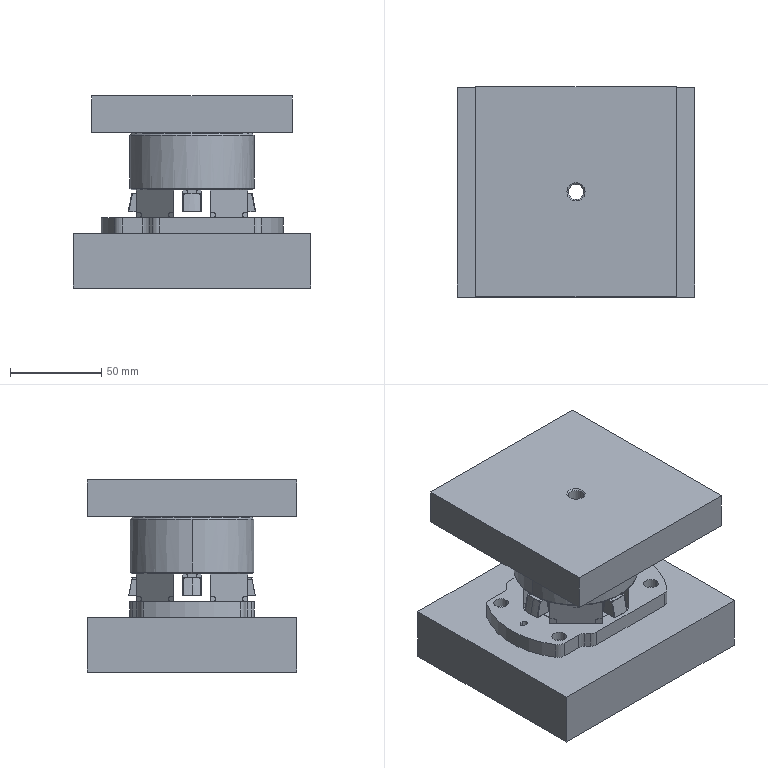Part | 4 solids | 369 faces | box 130 x 115 x 105.2 mm | volume 839123 mm3 | cylinder 152 | plane 152 | cone 65 | commonest cylinder face diameters 2 x24 2.4 x16 10 x16 4.5 x12 8 x12 54 x12